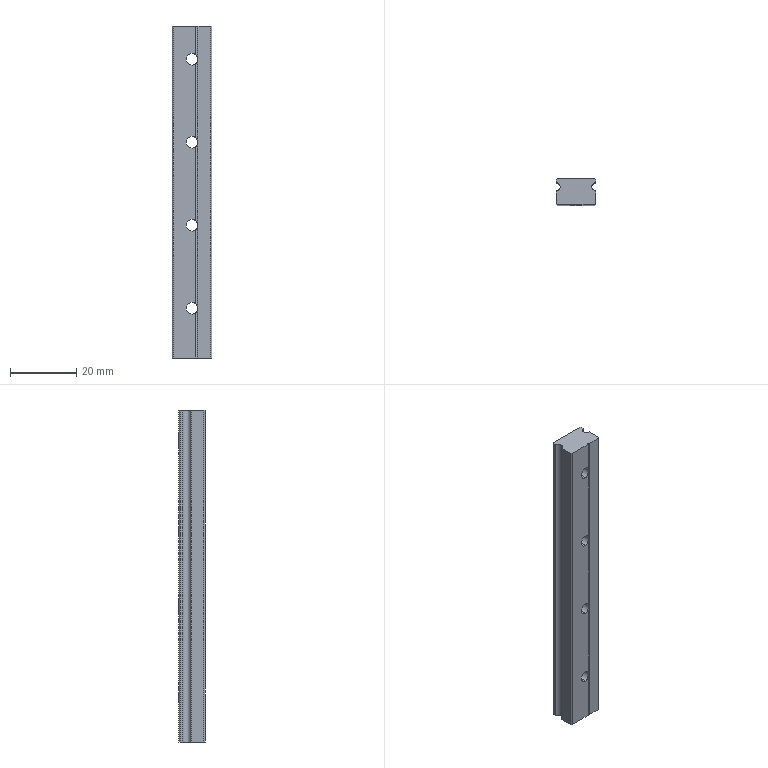Part | SolidWorks | features ICE 3, BaseBody 1 | 1 solid | 37 faces | box 12 x 8 x 100 mm | volume 8420 mm3 | cylinder 20 | plane 17 | commonest cylinder face diameters 3.5 x8 6 x8 2.5 x3 0.6 x1
STEP:
#1=CARTESIAN_POINT('',(0.,0.,-51.75));
#2=VERTEX_POINT('',#1);
#3=CARTESIAN_POINT('',(0.,0.,-48.25));
#4=VERTEX_POINT('',#3);
#5=CARTESIAN_POINT('',(0.,0.,-50.));
#6=DIRECTION('',(0.,1.,0.));
#7=DIRECTION('',(0.,0.,1.));
#8=AXIS2_PLACEMENT_3D('',#5,#6,#7);
#9=CIRCLE('',#8,1.75);
#10=EDGE_CURVE('',#2,#4,#9,.T.);
#11=ORIENTED_EDGE('',*,*,#10,.F.);
#12=CARTESIAN_POINT('',(0.,3.5,-51.75));
#13=VERTEX_POINT('',#12);
#14=CARTESIAN_POINT('',(0.,-0.006662,-51.75));
#15=DIRECTION('',(0.,1.,0.));
#16=VECTOR('',#15,1000.);
#17=LINE('',#14,#16);
#18=EDGE_CURVE('',#2,#13,#17,.T.);
#19=ORIENTED_EDGE('',*,*,#18,.T.);
#20=CARTESIAN_POINT('',(0.,3.5,-48.25));
#21=VERTEX_POINT('',#20);
#22=CARTESIAN_POINT('',(0.,3.5,-50.));
#23=DIRECTION('',(0.,1.,0.));
#24=DIRECTION('',(0.,0.,1.));
#25=AXIS2_PLACEMENT_3D('',#22,#23,#24);
#26=CIRCLE('',#25,1.75);
#27=EDGE_CURVE('',#13,#21,#26,.T.);
#28=ORIENTED_EDGE('',*,*,#27,.T.);
#29=CARTESIAN_POINT('',(0.,-0.006662,-48.25));
#30=DIRECTION('',(0.,1.,0.));
#31=VECTOR('',#30,1000.);
#32=LINE('',#29,#31);
#33=EDGE_CURVE('',#4,#21,#32,.T.);
#34=ORIENTED_EDGE('',*,*,#33,.F.);
#35=EDGE_LOOP('',(#11,#19,#28,#34));
#36=FACE_OUTER_BOUND('',#35,.T.);
#37=CARTESIAN_POINT('',(0.,-0.006662,-50.));
#38=DIRECTION('',(0.,1.,0.));
#39=DIRECTION('',(0.,0.,1.));
#40=AXIS2_PLACEMENT_3D('',#37,#38,#39);
#41=CYLINDRICAL_SURFACE('',#40,1.75);
#42=ADVANCED_FACE('',(#36),#41,.F.);
#43=CARTESIAN_POINT('',(0.,3.5,-53.));
#44=VERTEX_POINT('',#43);
#45=CARTESIAN_POINT('',(0.,3.5,-47.));
#46=VERTEX_POINT('',#45);
#47=CARTESIAN_POINT('',(0.,3.5,-50.));
#48=DIRECTION('',(0.,1.,0.));
#49=DIRECTION('',(0.,0.,1.));
#50=AXIS2_PLACEMENT_3D('',#47,#48,#49);
#51=CIRCLE('',#50,3.);
#52=EDGE_CURVE('',#44,#46,#51,.T.);
#53=ORIENTED_EDGE('',*,*,#52,.F.);
#54=CARTESIAN_POINT('',(0.,8.,-53.));
#55=VERTEX_POINT('',#54);
#56=CARTESIAN_POINT('',(0.,3.5,-53.));
#57=DIRECTION('',(0.,1.,0.));
#58=VECTOR('',#57,1000.);
#59=LINE('',#56,#58);
#60=EDGE_CURVE('',#44,#55,#59,.T.);
#61=ORIENTED_EDGE('',*,*,#60,.T.);
#62=CARTESIAN_POINT('',(0.,8.,-47.));
#63=VERTEX_POINT('',#62);
#64=CARTESIAN_POINT('',(0.,8.,-50.));
#65=DIRECTION('',(0.,1.,0.));
#66=DIRECTION('',(0.,0.,1.));
#67=AXIS2_PLACEMENT_3D('',#64,#65,#66);
#68=CIRCLE('',#67,3.);
#69=EDGE_CURVE('',#55,#63,#68,.T.);
#70=ORIENTED_EDGE('',*,*,#69,.T.);
#71=CARTESIAN_POINT('',(0.,3.5,-47.));
#72=DIRECTION('',(0.,1.,0.));
#73=VECTOR('',#72,1000.);
#74=LINE('',#71,#73);
#75=EDGE_CURVE('',#46,#63,#74,.T.);
#76=ORIENTED_EDGE('',*,*,#75,.F.);
#77=EDGE_LOOP('',(#53,#61,#70,#76));
#78=FACE_OUTER_BOUND('',#77,.T.);
#79=CARTESIAN_POINT('',(0.,3.5,-50.));
#80=DIRECTION('',(0.,1.,0.));
#81=DIRECTION('',(0.,0.,1.));
#82=AXIS2_PLACEMENT_3D('',#79,#80,#81);
#83=CYLINDRICAL_SURFACE('',#82,3.);
#84=ADVANCED_FACE('',(#78),#83,.F.);
#85=CARTESIAN_POINT('',(0.,3.5,1.75));
#86=VERTEX_POINT('',#85);
#87=CARTESIAN_POINT('',(0.,3.5,-1.75));
#88=VERTEX_POINT('',#87);
#89=CARTESIAN_POINT('',(0.,3.5,0.));
#90=DIRECTION('',(0.,-1.,0.));
#91=DIRECTION('',(0.,0.,-1.));
#92=AXIS2_PLACEMENT_3D('',#89,#90,#91);
#93=CIRCLE('',#92,1.75);
#94=EDGE_CURVE('',#86,#88,#93,.T.);
#95=ORIENTED_EDGE('',*,*,#94,.F.);
#96=CARTESIAN_POINT('',(0.,0.,1.75));
#97=VERTEX_POINT('',#96);
#98=CARTESIAN_POINT('',(0.,-8.977,1.75));
#99=DIRECTION('',(0.,-1.,0.));
#100=VECTOR('',#99,1000.);
#101=LINE('',#98,#100);
#102=EDGE_CURVE('',#86,#97,#101,.T.);
#103=ORIENTED_EDGE('',*,*,#102,.T.);
#104=CARTESIAN_POINT('',(0.,0.,-1.75));
#105=VERTEX_POINT('',#104);
#106=CARTESIAN_POINT('',(0.,0.,0.));
#107=DIRECTION('',(0.,1.,0.));
#108=DIRECTION('',(0.,0.,1.));
#109=AXIS2_PLACEMENT_3D('',#106,#107,#108);
#110=CIRCLE('',#109,1.75);
#111=EDGE_CURVE('',#105,#97,#110,.T.);
#112=ORIENTED_EDGE('',*,*,#111,.F.);
#113=CARTESIAN_POINT('',(0.,-8.977,-1.75));
#114=DIRECTION('',(0.,-1.,0.));
#115=VECTOR('',#114,1000.);
#116=LINE('',#113,#115);
#117=EDGE_CURVE('',#88,#105,#116,.T.);
#118=ORIENTED_EDGE('',*,*,#117,.F.);
#119=EDGE_LOOP('',(#95,#103,#112,#118));
#120=FACE_OUTER_BOUND('',#119,.T.);
#121=CARTESIAN_POINT('',(0.,-8.977,0.));
#122=DIRECTION('',(0.,-1.,0.));
#123=DIRECTION('',(0.,0.,-1.));
#124=AXIS2_PLACEMENT_3D('',#121,#122,#123);
#125=CYLINDRICAL_SURFACE('',#124,1.75);
#126=ADVANCED_FACE('',(#120),#125,.F.);
#127=CARTESIAN_POINT('',(0.,8.,28.));
#128=VERTEX_POINT('',#127);
#129=CARTESIAN_POINT('',(0.,8.,22.));
#130=VERTEX_POINT('',#129);
#131=CARTESIAN_POINT('',(0.,8.,25.));
#132=DIRECTION('',(0.,-1.,0.));
#133=DIRECTION('',(0.,0.,-1.));
#134=AXIS2_PLACEMENT_3D('',#131,#132,#133);
#135=CIRCLE('',#134,3.);
#136=EDGE_CURVE('',#128,#130,#135,.T.);
#137=ORIENTED_EDGE('',*,*,#136,.F.);
#138=CARTESIAN_POINT('',(0.,3.5,28.));
#139=VERTEX_POINT('',#138);
#140=CARTESIAN_POINT('',(0.,8.,28.));
#141=DIRECTION('',(0.,-1.,0.));
#142=VECTOR('',#141,1000.);
#143=LINE('',#140,#142);
#144=EDGE_CURVE('',#128,#139,#143,.T.);
#145=ORIENTED_EDGE('',*,*,#144,.T.);
#146=CARTESIAN_POINT('',(0.,3.5,22.));
#147=VERTEX_POINT('',#146);
#148=CARTESIAN_POINT('',(0.,3.5,25.));
#149=DIRECTION('',(0.,1.,0.));
#150=DIRECTION('',(-1.,0.,0.));
#151=AXIS2_PLACEMENT_3D('',#148,#149,#150);
#152=CIRCLE('',#151,3.);
#153=EDGE_CURVE('',#147,#139,#152,.T.);
#154=ORIENTED_EDGE('',*,*,#153,.F.);
#155=CARTESIAN_POINT('',(0.,8.,22.));
#156=DIRECTION('',(0.,-1.,0.));
#157=VECTOR('',#156,1000.);
#158=LINE('',#155,#157);
#159=EDGE_CURVE('',#130,#147,#158,.T.);
#160=ORIENTED_EDGE('',*,*,#159,.F.);
#161=EDGE_LOOP('',(#137,#145,#154,#160));
#162=FACE_OUTER_BOUND('',#161,.T.);
#163=CARTESIAN_POINT('',(0.,8.,25.));
#164=DIRECTION('',(0.,-1.,0.));
#165=DIRECTION('',(0.,0.,-1.));
#166=AXIS2_PLACEMENT_3D('',#163,#164,#165);
#167=CYLINDRICAL_SURFACE('',#166,3.);
#168=ADVANCED_FACE('',(#162),#167,.F.);
#169=CARTESIAN_POINT('',(4.75,5.5,35.));
#170=VERTEX_POINT('',#169);
#171=CARTESIAN_POINT('',(6.,6.75,35.));
#172=VERTEX_POINT('',#171);
#173=CARTESIAN_POINT('',(6.,5.5,35.));
#174=DIRECTION('',(0.,0.,-1.));
#175=DIRECTION('',(0.,-1.,0.));
#176=AXIS2_PLACEMENT_3D('',#173,#174,#175);
#177=CIRCLE('',#176,1.25);
#178=EDGE_CURVE('',#170,#172,#177,.T.);
#179=ORIENTED_EDGE('',*,*,#178,.F.);
#180=CARTESIAN_POINT('',(4.75,5.5,-65.));
#181=VERTEX_POINT('',#180);
#182=CARTESIAN_POINT('',(4.75,5.5,35.));
#183=DIRECTION('',(0.,0.,-1.));
#184=VECTOR('',#183,1000.);
#185=LINE('',#182,#184);
#186=EDGE_CURVE('',#170,#181,#185,.T.);
#187=ORIENTED_EDGE('',*,*,#186,.T.);
#188=CARTESIAN_POINT('',(6.,6.75,-65.));
#189=VERTEX_POINT('',#188);
#190=CARTESIAN_POINT('',(6.,5.5,-65.));
#191=DIRECTION('',(0.,0.,1.));
#192=DIRECTION('',(-1.,0.,0.));
#193=AXIS2_PLACEMENT_3D('',#190,#191,#192);
#194=CIRCLE('',#193,1.25);
#195=EDGE_CURVE('',#189,#181,#194,.T.);
#196=ORIENTED_EDGE('',*,*,#195,.F.);
#197=CARTESIAN_POINT('',(6.,6.75,-35.));
#198=DIRECTION('',(0.,0.,1.));
#199=VECTOR('',#198,1000.);
#200=LINE('',#197,#199);
#201=EDGE_CURVE('',#189,#172,#200,.T.);
#202=ORIENTED_EDGE('',*,*,#201,.T.);
#203=EDGE_LOOP('',(#179,#187,#196,#202));
#204=FACE_OUTER_BOUND('',#203,.T.);
#205=CARTESIAN_POINT('',(6.,5.5,35.));
#206=DIRECTION('',(0.,0.,-1.));
#207=DIRECTION('',(-1.,0.,0.));
#208=AXIS2_PLACEMENT_3D('',#205,#206,#207);
#209=CYLINDRICAL_SURFACE('',#208,1.25);
#210=ADVANCED_FACE('',(#204),#209,.F.);
#211=CARTESIAN_POINT('',(0.,8.,-22.));
#212=VERTEX_POINT('',#211);
#213=CARTESIAN_POINT('',(0.,8.,-28.));
#214=VERTEX_POINT('',#213);
#215=CARTESIAN_POINT('',(0.,8.,-25.));
#216=DIRECTION('',(0.,-1.,0.));
#217=DIRECTION('',(0.,0.,-1.));
#218=AXIS2_PLACEMENT_3D('',#215,#216,#217);
#219=CIRCLE('',#218,3.);
#220=EDGE_CURVE('',#212,#214,#219,.T.);
#221=ORIENTED_EDGE('',*,*,#220,.F.);
#222=CARTESIAN_POINT('',(0.,3.5,-22.));
#223=VERTEX_POINT('',#222);
#224=CARTESIAN_POINT('',(0.,8.,-22.));
#225=DIRECTION('',(0.,-1.,0.));
#226=VECTOR('',#225,1000.);
#227=LINE('',#224,#226);
#228=EDGE_CURVE('',#212,#223,#227,.T.);
#229=ORIENTED_EDGE('',*,*,#228,.T.);
#230=CARTESIAN_POINT('',(0.,3.5,-28.));
#231=VERTEX_POINT('',#230);
#232=CARTESIAN_POINT('',(0.,3.5,-25.));
#233=DIRECTION('',(0.,1.,0.));
#234=DIRECTION('',(-1.,0.,0.));
#235=AXIS2_PLACEMENT_3D('',#232,#233,#234);
#236=CIRCLE('',#235,3.);
#237=EDGE_CURVE('',#231,#223,#236,.T.);
#238=ORIENTED_EDGE('',*,*,#237,.F.);
#239=CARTESIAN_POINT('',(0.,8.,-28.));
#240=DIRECTION('',(0.,-1.,0.));
#241=VECTOR('',#240,1000.);
#242=LINE('',#239,#241);
#243=EDGE_CURVE('',#214,#231,#242,.T.);
#244=ORIENTED_EDGE('',*,*,#243,.F.);
#245=EDGE_LOOP('',(#221,#229,#238,#244));
#246=FACE_OUTER_BOUND('',#245,.T.);
#247=CARTESIAN_POINT('',(0.,8.,-25.));
#248=DIRECTION('',(0.,-1.,0.));
#249=DIRECTION('',(0.,0.,-1.));
#250=AXIS2_PLACEMENT_3D('',#247,#248,#249);
#251=CYLINDRICAL_SURFACE('',#250,3.);
#252=ADVANCED_FACE('',(#246),#251,.F.);
#253=CARTESIAN_POINT('',(0.,8.,3.));
#254=VERTEX_POINT('',#253);
#255=CARTESIAN_POINT('',(0.,8.,-3.));
#256=VERTEX_POINT('',#255);
#257=CARTESIAN_POINT('',(0.,8.,0.));
#258=DIRECTION('',(0.,-1.,0.));
#259=DIRECTION('',(0.,0.,-1.));
#260=AXIS2_PLACEMENT_3D('',#257,#258,#259);
#261=CIRCLE('',#260,3.);
#262=EDGE_CURVE('',#254,#256,#261,.T.);
#263=ORIENTED_EDGE('',*,*,#262,.F.);
#264=CARTESIAN_POINT('',(0.,3.5,3.));
#265=VERTEX_POINT('',#264);
#266=CARTESIAN_POINT('',(0.,8.,3.));
#267=DIRECTION('',(0.,-1.,0.));
#268=VECTOR('',#267,1000.);
#269=LINE('',#266,#268);
#270=EDGE_CURVE('',#254,#265,#269,.T.);
#271=ORIENTED_EDGE('',*,*,#270,.T.);
#272=CARTESIAN_POINT('',(0.,3.5,-3.));
#273=VERTEX_POINT('',#272);
#274=CARTESIAN_POINT('',(0.,3.5,0.));
#275=DIRECTION('',(0.,1.,0.));
#276=DIRECTION('',(-1.,0.,0.));
#277=AXIS2_PLACEMENT_3D('',#274,#275,#276);
#278=CIRCLE('',#277,3.);
#279=EDGE_CURVE('',#273,#265,#278,.T.);
#280=ORIENTED_EDGE('',*,*,#279,.F.);
#281=CARTESIAN_POINT('',(0.,8.,-3.));
#282=DIRECTION('',(0.,-1.,0.));
#283=VECTOR('',#282,1000.);
#284=LINE('',#281,#283);
#285=EDGE_CURVE('',#256,#273,#284,.T.);
#286=ORIENTED_EDGE('',*,*,#285,.F.);
#287=EDGE_LOOP('',(#263,#271,#280,#286));
#288=FACE_OUTER_BOUND('',#287,.T.);
#289=CARTESIAN_POINT('',(0.,8.,0.));
#290=DIRECTION('',(0.,-1.,0.));
#291=DIRECTION('',(0.,0.,-1.));
#292=AXIS2_PLACEMENT_3D('',#289,#290,#291);
#293=CYLINDRICAL_SURFACE('',#292,3.);
#294=ADVANCED_FACE('',(#288),#293,.F.);
#295=CARTESIAN_POINT('',(0.,3.5,26.75));
#296=VERTEX_POINT('',#295);
#297=CARTESIAN_POINT('',(0.,3.5,23.25));
#298=VERTEX_POINT('',#297);
#299=CARTESIAN_POINT('',(0.,3.5,25.));
#300=DIRECTION('',(0.,-1.,0.));
#301=DIRECTION('',(0.,0.,-1.));
#302=AXIS2_PLACEMENT_3D('',#299,#300,#301);
#303=CIRCLE('',#302,1.75);
#304=EDGE_CURVE('',#296,#298,#303,.T.);
#305=ORIENTED_EDGE('',*,*,#304,.F.);
#306=CARTESIAN_POINT('',(0.,0.,26.75));
#307=VERTEX_POINT('',#306);
#308=CARTESIAN_POINT('',(0.,-8.977,26.75));
#309=DIRECTION('',(0.,-1.,0.));
#310=VECTOR('',#309,1000.);
#311=LINE('',#308,#310);
#312=EDGE_CURVE('',#296,#307,#311,.T.);
#313=ORIENTED_EDGE('',*,*,#312,.T.);
#314=CARTESIAN_POINT('',(0.,0.,23.25));
#315=VERTEX_POINT('',#314);
#316=CARTESIAN_POINT('',(0.,0.,25.));
#317=DIRECTION('',(0.,1.,0.));
#318=DIRECTION('',(0.,0.,1.));
#319=AXIS2_PLACEMENT_3D('',#316,#317,#318);
#320=CIRCLE('',#319,1.75);
#321=EDGE_CURVE('',#315,#307,#320,.T.);
#322=ORIENTED_EDGE('',*,*,#321,.F.);
#323=CARTESIAN_POINT('',(0.,-8.977,23.25));
#324=DIRECTION('',(0.,-1.,0.));
#325=VECTOR('',#324,1000.);
#326=LINE('',#323,#325);
#327=EDGE_CURVE('',#298,#315,#326,.T.);
#328=ORIENTED_EDGE('',*,*,#327,.F.);
#329=EDGE_LOOP('',(#305,#313,#322,#328));
#330=FACE_OUTER_BOUND('',#329,.T.);
#331=CARTESIAN_POINT('',(0.,-8.977,25.));
#332=DIRECTION('',(0.,-1.,0.));
#333=DIRECTION('',(0.,0.,-1.));
#334=AXIS2_PLACEMENT_3D('',#331,#332,#333);
#335=CYLINDRICAL_SURFACE('',#334,1.75);
#336=ADVANCED_FACE('',(#330),#335,.F.);
#337=CARTESIAN_POINT('',(0.,3.5,-23.25));
#338=VERTEX_POINT('',#337);
#339=CARTESIAN_POINT('',(0.,3.5,-26.75));
#340=VERTEX_POINT('',#339);
#341=CARTESIAN_POINT('',(0.,3.5,-25.));
#342=DIRECTION('',(0.,-1.,0.));
#343=DIRECTION('',(0.,0.,-1.));
#344=AXIS2_PLACEMENT_3D('',#341,#342,#343);
#345=CIRCLE('',#344,1.75);
#346=EDGE_CURVE('',#338,#340,#345,.T.);
#347=ORIENTED_EDGE('',*,*,#346,.F.);
#348=CARTESIAN_POINT('',(0.,0.,-23.25));
#349=VERTEX_POINT('',#348);
#350=CARTESIAN_POINT('',(0.,-8.977,-23.25));
#351=DIRECTION('',(0.,-1.,0.));
#352=VECTOR('',#351,1000.);
#353=LINE('',#350,#352);
#354=EDGE_CURVE('',#338,#349,#353,.T.);
#355=ORIENTED_EDGE('',*,*,#354,.T.);
#356=CARTESIAN_POINT('',(0.,0.,-26.75));
#357=VERTEX_POINT('',#356);
#358=CARTESIAN_POINT('',(0.,0.,-25.));
#359=DIRECTION('',(0.,1.,0.));
#360=DIRECTION('',(0.,0.,1.));
#361=AXIS2_PLACEMENT_3D('',#358,#359,#360);
#362=CIRCLE('',#361,1.75);
#363=EDGE_CURVE('',#357,#349,#362,.T.);
#364=ORIENTED_EDGE('',*,*,#363,.F.);
#365=CARTESIAN_POINT('',(0.,-8.977,-26.75));
#366=DIRECTION('',(0.,-1.,0.));
#367=VECTOR('',#366,1000.);
#368=LINE('',#365,#367);
#369=EDGE_CURVE('',#340,#357,#368,.T.);
#370=ORIENTED_EDGE('',*,*,#369,.F.);
#371=EDGE_LOOP('',(#347,#355,#364,#370));
#372=FACE_OUTER_BOUND('',#371,.T.);
#373=CARTESIAN_POINT('',(0.,-8.977,-25.));
#374=DIRECTION('',(0.,-1.,0.));
#375=DIRECTION('',(0.,0.,-1.));
#376=AXIS2_PLACEMENT_3D('',#373,#374,#375);
#377=CYLINDRICAL_SURFACE('',#376,1.75);
#378=ADVANCED_FACE('',(#372),#377,.F.);
#379=ORIENTED_EDGE('',*,*,#354,.F.);
#380=CARTESIAN_POINT('',(0.,3.5,-25.));
#381=DIRECTION('',(0.,-1.,0.));
#382=DIRECTION('',(0.,0.,-1.));
#383=AXIS2_PLACEMENT_3D('',#380,#381,#382);
#384=CIRCLE('',#383,1.75);
#385=EDGE_CURVE('',#340,#338,#384,.T.);
#386=ORIENTED_EDGE('',*,*,#385,.F.);
#387=ORIENTED_EDGE('',*,*,#369,.T.);
#388=CARTESIAN_POINT('',(1.2,0.,-26.274));
#389=VERTEX_POINT('',#388);
#390=CARTESIAN_POINT('',(0.,0.,-25.));
#391=DIRECTION('',(0.,1.,0.));
#392=DIRECTION('',(0.,0.,1.));
#393=AXIS2_PLACEMENT_3D('',#390,#391,#392);
#394=CIRCLE('',#393,1.75);
#395=EDGE_CURVE('',#389,#357,#394,.T.);
#396=ORIENTED_EDGE('',*,*,#395,.F.);
#397=CARTESIAN_POINT('',(1.2,0.,-23.726));
#398=VERTEX_POINT('',#397);
#399=CARTESIAN_POINT('',(1.2,0.,-26.274));
#400=CARTESIAN_POINT('',(1.2,0.02075,-26.274));
#401=CARTESIAN_POINT('',(1.202,0.04091,-26.272));
#402=CARTESIAN_POINT('',(1.21,0.08005,-26.264));
#403=CARTESIAN_POINT('',(1.216,0.09786,-26.259));
#404=CARTESIAN_POINT('',(1.241,0.1565,-26.234));
#405=CARTESIAN_POINT('',(1.265,0.1906,-26.21));
#406=CARTESIAN_POINT('',(1.321,0.2436,-26.149));
#407=CARTESIAN_POINT('',(1.352,0.2638,-26.112));
#408=CARTESIAN_POINT('',(1.403,0.2845,-26.047));
#409=CARTESIAN_POINT('',(1.42,0.2898,-26.023));
#410=CARTESIAN_POINT('',(1.446,0.2954,-25.985));
#411=CARTESIAN_POINT('',(1.46,0.2976,-25.966));
#412=CARTESIAN_POINT('',(1.473,0.2988,-25.945));
#413=CARTESIAN_POINT('',(1.482,0.2995,-25.931));
#414=CARTESIAN_POINT('',(1.488,0.2998,-25.922));
#415=CARTESIAN_POINT('',(1.52,0.3007,-25.87));
#416=CARTESIAN_POINT('',(1.55,0.2969,-25.815));
#417=CARTESIAN_POINT('',(1.595,0.2843,-25.72));
#418=CARTESIAN_POINT('',(1.61,0.2789,-25.686));
#419=CARTESIAN_POINT('',(1.639,0.2659,-25.613));
#420=CARTESIAN_POINT('',(1.654,0.2578,-25.573));
#421=CARTESIAN_POINT('',(1.679,0.241,-25.494));
#422=CARTESIAN_POINT('',(1.696,0.2284,-25.435));
#423=CARTESIAN_POINT('',(1.709,0.2156,-25.375));
#424=CARTESIAN_POINT('',(1.718,0.2071,-25.335));
#425=CARTESIAN_POINT('',(1.721,0.2032,-25.317));
#426=CARTESIAN_POINT('',(1.733,0.1892,-25.25));
#427=CARTESIAN_POINT('',(1.741,0.1782,-25.183));
#428=CARTESIAN_POINT('',(1.746,0.1718,-25.116));
#429=CARTESIAN_POINT('',(1.749,0.1686,-25.071));
#430=CARTESIAN_POINT('',(1.749,0.1674,-25.047));
#431=CARTESIAN_POINT('',(1.75,0.1657,-24.985));
#432=CARTESIAN_POINT('',(1.75,0.167,-24.941));
#433=CARTESIAN_POINT('',(1.746,0.1726,-24.873));
#434=CARTESIAN_POINT('',(1.743,0.1762,-24.839));
#435=CARTESIAN_POINT('',(1.738,0.1821,-24.797));
#436=CARTESIAN_POINT('',(1.736,0.1854,-24.776));
#437=CARTESIAN_POINT('',(1.734,0.187,-24.767));
#438=CARTESIAN_POINT('',(1.734,0.188,-24.761));
#439=CARTESIAN_POINT('',(1.733,0.1889,-24.756));
#440=CARTESIAN_POINT('',(1.73,0.192,-24.738));
#441=CARTESIAN_POINT('',(1.726,0.1978,-24.709));
#442=CARTESIAN_POINT('',(1.714,0.2107,-24.646));
#443=CARTESIAN_POINT('',(1.709,0.2157,-24.623));
#444=CARTESIAN_POINT('',(1.699,0.2243,-24.582));
#445=CARTESIAN_POINT('',(1.694,0.2289,-24.561));
#446=CARTESIAN_POINT('',(1.687,0.2347,-24.534));
#447=CARTESIAN_POINT('',(1.684,0.2373,-24.522));
#448=CARTESIAN_POINT('',(1.681,0.239,-24.514));
#449=CARTESIAN_POINT('',(1.68,0.2402,-24.509));
#450=CARTESIAN_POINT('',(1.653,0.2604,-24.417));
#451=CARTESIAN_POINT('',(1.622,0.2752,-24.339));
#452=CARTESIAN_POINT('',(1.576,0.29,-24.238));
#453=CARTESIAN_POINT('',(1.56,0.2937,-24.207));
#454=CARTESIAN_POINT('',(1.538,0.2974,-24.164));
#455=CARTESIAN_POINT('',(1.526,0.2988,-24.144));
#456=CARTESIAN_POINT('',(1.515,0.2996,-24.125));
#457=CARTESIAN_POINT('',(1.508,0.2999,-24.112));
#458=CARTESIAN_POINT('',(1.506,0.3,-24.108));
#459=CARTESIAN_POINT('',(1.464,0.3001,-24.039));
#460=CARTESIAN_POINT('',(1.427,0.2936,-23.986));
#461=CARTESIAN_POINT('',(1.358,0.2669,-23.894));
#462=CARTESIAN_POINT('',(1.326,0.2475,-23.857));
#463=CARTESIAN_POINT('',(1.281,0.2065,-23.808));
#464=CARTESIAN_POINT('',(1.268,0.1912,-23.794));
#465=CARTESIAN_POINT('',(1.244,0.1575,-23.769));
#466=CARTESIAN_POINT('',(1.233,0.1376,-23.758));
#467=CARTESIAN_POINT('',(1.208,0.08193,-23.734));
#468=CARTESIAN_POINT('',(1.2,0.04225,-23.726));
#469=CARTESIAN_POINT('',(1.2,0.,-23.726));
#470=B_SPLINE_CURVE_WITH_KNOTS('',3,(#399,#400,#401,#402,#403,#404,#405,#406,#407,#408,#409,#410,#411,#412,#413,#414,#415,#416,#417,#418,#419,#420,#421,#422,#423,#424,#425,#426,#427,#428,#429,#430,#431,#432,#433,#434,#435,#436,#437,#438,#439,#440,#441,#442,#443,#444,#445,#446,#447,#448,#449,#450,#451,#452,#453,#454,#455,#456,#457,#458,#459,#460,#461,#462,#463,#464,#465,#466,#467,#468,#469),.UNSPECIFIED.,.F.,.F.,(4,2,2,2,2,2,1,2,2,2,2,2,1,2,2,1,2,2,2,1,1,1,2,2,2,2,1,1,2,2,2,2,1,2,2,2,2,2,2,4),(0.,0.03125,0.0625,0.125,0.1875,0.2187,0.2344,0.2422,0.25,0.3125,0.3437,0.375,0.4062,0.4219,0.4375,0.4687,0.4844,0.5,0.5312,0.5469,0.5547,0.5586,0.5605,0.5625,0.5937,0.6094,0.6172,0.6211,0.623,0.625,0.6875,0.7187,0.7344,0.7422,0.75,0.8125,0.875,0.9062,0.9375,1.),.UNSPECIFIED.);
#471=EDGE_CURVE('',#389,#398,#470,.T.);
#472=ORIENTED_EDGE('',*,*,#471,.T.);
#473=CARTESIAN_POINT('',(0.,0.,-25.));
#474=DIRECTION('',(0.,1.,0.));
#475=DIRECTION('',(0.,0.,1.));
#476=AXIS2_PLACEMENT_3D('',#473,#474,#475);
#477=CIRCLE('',#476,1.75);
#478=EDGE_CURVE('',#349,#398,#477,.T.);
#479=ORIENTED_EDGE('',*,*,#478,.F.);
#480=EDGE_LOOP('',(#379,#386,#387,#396,#472,#479));
#481=FACE_OUTER_BOUND('',#480,.T.);
#482=CARTESIAN_POINT('',(0.,-8.977,-25.));
#483=DIRECTION('',(0.,-1.,0.));
#484=DIRECTION('',(0.,0.,-1.));
#485=AXIS2_PLACEMENT_3D('',#482,#483,#484);
#486=CYLINDRICAL_SURFACE('',#485,1.75);
#487=ADVANCED_FACE('',(#481),#486,.F.);
#488=ORIENTED_EDGE('',*,*,#312,.F.);
#489=CARTESIAN_POINT('',(0.,3.5,25.));
#490=DIRECTION('',(0.,-1.,0.));
#491=DIRECTION('',(0.,0.,-1.));
#492=AXIS2_PLACEMENT_3D('',#489,#490,#491);
#493=CIRCLE('',#492,1.75);
#494=EDGE_CURVE('',#298,#296,#493,.T.);
#495=ORIENTED_EDGE('',*,*,#494,.F.);
#496=ORIENTED_EDGE('',*,*,#327,.T.);
#497=CARTESIAN_POINT('',(1.2,0.,23.726));
#498=VERTEX_POINT('',#497);
#499=CARTESIAN_POINT('',(0.,0.,25.));
#500=DIRECTION('',(0.,1.,0.));
#501=DIRECTION('',(0.,0.,1.));
#502=AXIS2_PLACEMENT_3D('',#499,#500,#501);
#503=CIRCLE('',#502,1.75);
#504=EDGE_CURVE('',#498,#315,#503,.T.);
#505=ORIENTED_EDGE('',*,*,#504,.F.);
#506=CARTESIAN_POINT('',(1.2,0.,26.274));
#507=VERTEX_POINT('',#506);
#508=CARTESIAN_POINT('',(1.2,0.,23.726));
#509=CARTESIAN_POINT('',(1.2,0.02075,23.726));
#510=CARTESIAN_POINT('',(1.202,0.04091,23.728));
#511=CARTESIAN_POINT('',(1.21,0.08005,23.736));
#512=CARTESIAN_POINT('',(1.216,0.09786,23.741));
#513=CARTESIAN_POINT('',(1.241,0.1565,23.766));
#514=CARTESIAN_POINT('',(1.265,0.1906,23.79));
#515=CARTESIAN_POINT('',(1.321,0.2436,23.851));
#516=CARTESIAN_POINT('',(1.352,0.2638,23.888));
#517=CARTESIAN_POINT('',(1.403,0.2845,23.953));
#518=CARTESIAN_POINT('',(1.42,0.2898,23.977));
#519=CARTESIAN_POINT('',(1.446,0.2954,24.015));
#520=CARTESIAN_POINT('',(1.46,0.2976,24.034));
#521=CARTESIAN_POINT('',(1.473,0.2988,24.055));
#522=CARTESIAN_POINT('',(1.482,0.2995,24.069));
#523=CARTESIAN_POINT('',(1.488,0.2998,24.078));
#524=CARTESIAN_POINT('',(1.52,0.3007,24.13));
#525=CARTESIAN_POINT('',(1.55,0.2969,24.185));
#526=CARTESIAN_POINT('',(1.595,0.2843,24.28));
#527=CARTESIAN_POINT('',(1.61,0.2789,24.314));
#528=CARTESIAN_POINT('',(1.639,0.2659,24.387));
#529=CARTESIAN_POINT('',(1.654,0.2578,24.427));
#530=CARTESIAN_POINT('',(1.679,0.241,24.506));
#531=CARTESIAN_POINT('',(1.696,0.2284,24.565));
#532=CARTESIAN_POINT('',(1.709,0.2156,24.625));
#533=CARTESIAN_POINT('',(1.718,0.2071,24.665));
#534=CARTESIAN_POINT('',(1.721,0.2032,24.683));
#535=CARTESIAN_POINT('',(1.733,0.1892,24.75));
#536=CARTESIAN_POINT('',(1.741,0.1782,24.817));
#537=CARTESIAN_POINT('',(1.746,0.1718,24.884));
#538=CARTESIAN_POINT('',(1.749,0.1686,24.929));
#539=CARTESIAN_POINT('',(1.749,0.1674,24.953));
#540=CARTESIAN_POINT('',(1.75,0.1657,25.015));
#541=CARTESIAN_POINT('',(1.75,0.167,25.059));
#542=CARTESIAN_POINT('',(1.746,0.1726,25.127));
#543=CARTESIAN_POINT('',(1.743,0.1762,25.161));
#544=CARTESIAN_POINT('',(1.738,0.1821,25.203));
#545=CARTESIAN_POINT('',(1.736,0.1854,25.224));
#546=CARTESIAN_POINT('',(1.734,0.187,25.233));
#547=CARTESIAN_POINT('',(1.734,0.188,25.239));
#548=CARTESIAN_POINT('',(1.733,0.1889,25.244));
#549=CARTESIAN_POINT('',(1.73,0.192,25.262));
#550=CARTESIAN_POINT('',(1.726,0.1978,25.291));
#551=CARTESIAN_POINT('',(1.714,0.2107,25.354));
#552=CARTESIAN_POINT('',(1.709,0.2157,25.377));
#553=CARTESIAN_POINT('',(1.699,0.2243,25.418));
#554=CARTESIAN_POINT('',(1.694,0.2289,25.439));
#555=CARTESIAN_POINT('',(1.687,0.2347,25.466));
#556=CARTESIAN_POINT('',(1.684,0.2373,25.478));
#557=CARTESIAN_POINT('',(1.681,0.239,25.486));
#558=CARTESIAN_POINT('',(1.68,0.2402,25.491));
#559=CARTESIAN_POINT('',(1.653,0.2604,25.583));
#560=CARTESIAN_POINT('',(1.622,0.2752,25.661));
#561=CARTESIAN_POINT('',(1.576,0.29,25.762));
#562=CARTESIAN_POINT('',(1.56,0.2937,25.793));
#563=CARTESIAN_POINT('',(1.538,0.2974,25.836));
#564=CARTESIAN_POINT('',(1.526,0.2988,25.856));
#565=CARTESIAN_POINT('',(1.515,0.2996,25.875));
#566=CARTESIAN_POINT('',(1.508,0.2999,25.888));
#567=CARTESIAN_POINT('',(1.506,0.3,25.892));
#568=CARTESIAN_POINT('',(1.464,0.3001,25.961));
#569=CARTESIAN_POINT('',(1.427,0.2936,26.014));
#570=CARTESIAN_POINT('',(1.358,0.2669,26.106));
#571=CARTESIAN_POINT('',(1.326,0.2475,26.143));
#572=CARTESIAN_POINT('',(1.281,0.2065,26.192));
#573=CARTESIAN_POINT('',(1.268,0.1912,26.206));
#574=CARTESIAN_POINT('',(1.244,0.1575,26.231));
#575=CARTESIAN_POINT('',(1.233,0.1376,26.242));
#576=CARTESIAN_POINT('',(1.208,0.08193,26.266));
#577=CARTESIAN_POINT('',(1.2,0.04225,26.274));
#578=CARTESIAN_POINT('',(1.2,0.,26.274));
#579=B_SPLINE_CURVE_WITH_KNOTS('',3,(#508,#509,#510,#511,#512,#513,#514,#515,#516,#517,#518,#519,#520,#521,#522,#523,#524,#525,#526,#527,#528,#529,#530,#531,#532,#533,#534,#535,#536,#537,#538,#539,#540,#541,#542,#543,#544,#545,#546,#547,#548,#549,#550,#551,#552,#553,#554,#555,#556,#557,#558,#559,#560,#561,#562,#563,#564,#565,#566,#567,#568,#569,#570,#571,#572,#573,#574,#575,#576,#577,#578),.UNSPECIFIED.,.F.,.F.,(4,2,2,2,2,2,1,2,2,2,2,2,1,2,2,1,2,2,2,1,1,1,2,2,2,2,1,1,2,2,2,2,1,2,2,2,2,2,2,4),(0.,0.03125,0.0625,0.125,0.1875,0.2187,0.2344,0.2422,0.25,0.3125,0.3437,0.375,0.4062,0.4219,0.4375,0.4687,0.4844,0.5,0.5312,0.5469,0.5547,0.5586,0.5605,0.5625,0.5937,0.6094,0.6172,0.6211,0.623,0.625,0.6875,0.7187,0.7344,0.7422,0.75,0.8125,0.875,0.9062,0.9375,1.),.UNSPECIFIED.);
#580=EDGE_CURVE('',#498,#507,#579,.T.);
#581=ORIENTED_EDGE('',*,*,#580,.T.);
#582=CARTESIAN_POINT('',(0.,0.,25.));
#583=DIRECTION('',(0.,1.,0.));
#584=DIRECTION('',(0.,0.,1.));
#585=AXIS2_PLACEMENT_3D('',#582,#583,#584);
#586=CIRCLE('',#585,1.75);
#587=EDGE_CURVE('',#307,#507,#586,.T.);
#588=ORIENTED_EDGE('',*,*,#587,.F.);
#589=EDGE_LOOP('',(#488,#495,#496,#505,#581,#588));
#590=FACE_OUTER_BOUND('',#589,.T.);
#591=CARTESIAN_POINT('',(0.,-8.977,25.));
#592=DIRECTION('',(0.,-1.,0.));
#593=DIRECTION('',(0.,0.,-1.));
#594=AXIS2_PLACEMENT_3D('',#591,#592,#593);
#595=CYLINDRICAL_SURFACE('',#594,1.75);
#596=ADVANCED_FACE('',(#590),#595,.F.);
#597=ORIENTED_EDGE('',*,*,#270,.F.);
#598=CARTESIAN_POINT('',(0.,8.,0.));
#599=DIRECTION('',(0.,-1.,0.));
#600=DIRECTION('',(0.,0.,-1.));
#601=AXIS2_PLACEMENT_3D('',#598,#599,#600);
#602=CIRCLE('',#601,3.);
#603=EDGE_CURVE('',#256,#254,#602,.T.);
#604=ORIENTED_EDGE('',*,*,#603,.F.);
#605=ORIENTED_EDGE('',*,*,#285,.T.);
#606=CARTESIAN_POINT('',(0.,3.5,0.));
#607=DIRECTION('',(0.,1.,0.));
#608=DIRECTION('',(-1.,0.,0.));
#609=AXIS2_PLACEMENT_3D('',#606,#607,#608);
#610=CIRCLE('',#609,3.);
#611=EDGE_CURVE('',#265,#273,#610,.T.);
#612=ORIENTED_EDGE('',*,*,#611,.F.);
#613=EDGE_LOOP('',(#597,#604,#605,#612));
#614=FACE_OUTER_BOUND('',#613,.T.);
#615=CARTESIAN_POINT('',(0.,8.,0.));
#616=DIRECTION('',(0.,-1.,0.));
#617=DIRECTION('',(0.,0.,-1.));
#618=AXIS2_PLACEMENT_3D('',#615,#616,#617);
#619=CYLINDRICAL_SURFACE('',#618,3.);
#620=ADVANCED_FACE('',(#614),#619,.F.);
#621=ORIENTED_EDGE('',*,*,#228,.F.);
#622=CARTESIAN_POINT('',(0.,8.,-25.));
#623=DIRECTION('',(0.,-1.,0.));
#624=DIRECTION('',(0.,0.,-1.));
#625=AXIS2_PLACEMENT_3D('',#622,#623,#624);
#626=CIRCLE('',#625,3.);
#627=EDGE_CURVE('',#214,#212,#626,.T.);
#628=ORIENTED_EDGE('',*,*,#627,.F.);
#629=ORIENTED_EDGE('',*,*,#243,.T.);
#630=CARTESIAN_POINT('',(0.,3.5,-25.));
#631=DIRECTION('',(0.,1.,0.));
#632=DIRECTION('',(-1.,0.,0.));
#633=AXIS2_PLACEMENT_3D('',#630,#631,#632);
#634=CIRCLE('',#633,3.);
#635=EDGE_CURVE('',#223,#231,#634,.T.);
#636=ORIENTED_EDGE('',*,*,#635,.F.);
#637=EDGE_LOOP('',(#621,#628,#629,#636));
#638=FACE_OUTER_BOUND('',#637,.T.);
#639=CARTESIAN_POINT('',(0.,8.,-25.));
#640=DIRECTION('',(0.,-1.,0.));
#641=DIRECTION('',(0.,0.,-1.));
#642=AXIS2_PLACEMENT_3D('',#639,#640,#641);
#643=CYLINDRICAL_SURFACE('',#642,3.);
#644=ADVANCED_FACE('',(#638),#643,.F.);
#645=CARTESIAN_POINT('',(-6.,7.6,-65.));
#646=VERTEX_POINT('',#645);
#647=CARTESIAN_POINT('',(-6.,7.6,35.));
#648=VERTEX_POINT('',#647);
#649=CARTESIAN_POINT('',(-6.,7.6,-35.));
#650=DIRECTION('',(0.,0.,1.));
#651=VECTOR('',#650,1000.);
#652=LINE('',#649,#651);
#653=EDGE_CURVE('',#646,#648,#652,.T.);
#654=ORIENTED_EDGE('',*,*,#653,.F.);
#655=CARTESIAN_POINT('',(-6.,6.75,-65.));
#656=VERTEX_POINT('',#655);
#657=CARTESIAN_POINT('',(-6.,6.75,-65.));
#658=DIRECTION('',(0.,1.,0.));
#659=VECTOR('',#658,1000.);
#660=LINE('',#657,#659);
#661=EDGE_CURVE('',#656,#646,#660,.T.);
#662=ORIENTED_EDGE('',*,*,#661,.F.);
#663=CARTESIAN_POINT('',(-6.,6.75,35.));
#664=VERTEX_POINT('',#663);
#665=CARTESIAN_POINT('',(-6.,6.75,35.));
#666=DIRECTION('',(0.,0.,-1.));
#667=VECTOR('',#666,1000.);
#668=LINE('',#665,#667);
#669=EDGE_CURVE('',#664,#656,#668,.T.);
#670=ORIENTED_EDGE('',*,*,#669,.F.);
#671=CARTESIAN_POINT('',(-6.,6.75,35.));
#672=DIRECTION('',(0.,1.,0.));
#673=VECTOR('',#672,1000.);
#674=LINE('',#671,#673);
#675=EDGE_CURVE('',#664,#648,#674,.T.);
#676=ORIENTED_EDGE('',*,*,#675,.T.);
#677=EDGE_LOOP('',(#654,#662,#670,#676));
#678=FACE_OUTER_BOUND('',#677,.T.);
#679=CARTESIAN_POINT('',(-6.,8.,35.));
#680=DIRECTION('',(1.,0.,0.));
#681=DIRECTION('',(0.,1.,0.));
#682=AXIS2_PLACEMENT_3D('',#679,#680,#681);
#683=PLANE('',#682);
#684=ADVANCED_FACE('',(#678),#683,.F.);
#685=CARTESIAN_POINT('',(-5.6,8.,35.));
#686=VERTEX_POINT('',#685);
#687=CARTESIAN_POINT('',(-5.6,8.,-65.));
#688=VERTEX_POINT('',#687);
#689=CARTESIAN_POINT('',(-5.6,8.,35.));
#690=DIRECTION('',(0.,0.,-1.));
#691=VECTOR('',#690,1000.);
#692=LINE('',#689,#691);
#693=EDGE_CURVE('',#686,#688,#692,.T.);
#694=ORIENTED_EDGE('',*,*,#693,.T.);
#695=CARTESIAN_POINT('',(-6.,7.6,-65.));
#696=DIRECTION('',(0.7071,0.7071,0.));
#697=VECTOR('',#696,1000.);
#698=LINE('',#695,#697);
#699=EDGE_CURVE('',#646,#688,#698,.T.);
#700=ORIENTED_EDGE('',*,*,#699,.F.);
#701=ORIENTED_EDGE('',*,*,#653,.T.);
#702=CARTESIAN_POINT('',(-5.6,8.,35.));
#703=DIRECTION('',(-0.7071,-0.7071,0.));
#704=VECTOR('',#703,1000.);
#705=LINE('',#702,#704);
#706=EDGE_CURVE('',#686,#648,#705,.T.);
#707=ORIENTED_EDGE('',*,*,#706,.F.);
#708=EDGE_LOOP('',(#694,#700,#701,#707));
#709=FACE_OUTER_BOUND('',#708,.T.);
#710=CARTESIAN_POINT('',(-6.,7.6,35.));
#711=DIRECTION('',(0.7071,-0.7071,0.));
#712=DIRECTION('',(0.,0.,-1.));
#713=AXIS2_PLACEMENT_3D('',#710,#711,#712);
#714=PLANE('',#713);
#715=ADVANCED_FACE('',(#709),#714,.F.);
#716=CARTESIAN_POINT('',(5.6,0.,35.));
#717=VERTEX_POINT('',#716);
#718=CARTESIAN_POINT('',(5.6,0.,-65.));
#719=VERTEX_POINT('',#718);
#720=CARTESIAN_POINT('',(5.6,0.,35.));
#721=DIRECTION('',(0.,0.,-1.));
#722=VECTOR('',#721,1000.);
#723=LINE('',#720,#722);
#724=EDGE_CURVE('',#717,#719,#723,.T.);
#725=ORIENTED_EDGE('',*,*,#724,.F.);
#726=CARTESIAN_POINT('',(1.8,0.,35.));
#727=VERTEX_POINT('',#726);
#728=CARTESIAN_POINT('',(5.6,0.,35.));
#729=DIRECTION('',(-1.,0.,0.));
#730=VECTOR('',#729,1000.);
#731=LINE('',#728,#730);
#732=EDGE_CURVE('',#717,#727,#731,.T.);
#733=ORIENTED_EDGE('',*,*,#732,.T.);
#734=CARTESIAN_POINT('',(1.8,0.,-65.));
#735=VERTEX_POINT('',#734);
#736=CARTESIAN_POINT('',(1.8,0.,-35.));
#737=DIRECTION('',(0.,0.,1.));
#738=VECTOR('',#737,1000.);
#739=LINE('',#736,#738);
#740=EDGE_CURVE('',#735,#727,#739,.T.);
#741=ORIENTED_EDGE('',*,*,#740,.F.);
#742=CARTESIAN_POINT('',(5.6,0.,-65.));
#743=DIRECTION('',(-1.,0.,0.));
#744=VECTOR('',#743,1000.);
#745=LINE('',#742,#744);
#746=EDGE_CURVE('',#719,#735,#745,.T.);
#747=ORIENTED_EDGE('',*,*,#746,.F.);
#748=EDGE_LOOP('',(#725,#733,#741,#747));
#749=FACE_OUTER_BOUND('',#748,.T.);
#750=CARTESIAN_POINT('',(1.8,0.,35.));
#751=DIRECTION('',(0.,1.,0.));
#752=DIRECTION('',(1.,0.,0.));
#753=AXIS2_PLACEMENT_3D('',#750,#751,#752);
#754=PLANE('',#753);
#755=ADVANCED_FACE('',(#749),#754,.F.);
#756=ORIENTED_EDGE('',*,*,#724,.T.);
#757=CARTESIAN_POINT('',(6.,0.4,-65.));
#758=VERTEX_POINT('',#757);
#759=CARTESIAN_POINT('',(6.,0.4,-65.));
#760=DIRECTION('',(-0.7071,-0.7071,0.));
#761=VECTOR('',#760,1000.);
#762=LINE('',#759,#761);
#763=EDGE_CURVE('',#758,#719,#762,.T.);
#764=ORIENTED_EDGE('',*,*,#763,.F.);
#765=CARTESIAN_POINT('',(6.,0.4,35.));
#766=VERTEX_POINT('',#765);
#767=CARTESIAN_POINT('',(6.,0.4,-35.));
#768=DIRECTION('',(0.,0.,1.));
#769=VECTOR('',#768,1000.);
#770=LINE('',#767,#769);
#771=EDGE_CURVE('',#758,#766,#770,.T.);
#772=ORIENTED_EDGE('',*,*,#771,.T.);
#773=CARTESIAN_POINT('',(5.6,0.,35.));
#774=DIRECTION('',(0.7071,0.7071,0.));
#775=VECTOR('',#774,1000.);
#776=LINE('',#773,#775);
#777=EDGE_CURVE('',#717,#766,#776,.T.);
#778=ORIENTED_EDGE('',*,*,#777,.F.);
#779=EDGE_LOOP('',(#756,#764,#772,#778));
#780=FACE_OUTER_BOUND('',#779,.T.);
#781=CARTESIAN_POINT('',(6.,0.4,35.));
#782=DIRECTION('',(-0.7071,0.7071,0.));
#783=DIRECTION('',(0.,0.,1.));
#784=AXIS2_PLACEMENT_3D('',#781,#782,#783);
#785=PLANE('',#784);
#786=ADVANCED_FACE('',(#780),#785,.F.);
#787=ORIENTED_EDGE('',*,*,#771,.F.);
#788=CARTESIAN_POINT('',(6.,4.25,-65.));
#789=VERTEX_POINT('',#788);
#790=CARTESIAN_POINT('',(6.,4.25,-65.));
#791=DIRECTION('',(0.,-1.,0.));
#792=VECTOR('',#791,1000.);
#793=LINE('',#790,#792);
#794=EDGE_CURVE('',#789,#758,#793,.T.);
#795=ORIENTED_EDGE('',*,*,#794,.F.);
#796=CARTESIAN_POINT('',(6.,4.25,35.));
#797=VERTEX_POINT('',#796);
#798=CARTESIAN_POINT('',(6.,4.25,35.));
#799=DIRECTION('',(0.,0.,-1.));
#800=VECTOR('',#799,1000.);
#801=LINE('',#798,#800);
#802=EDGE_CURVE('',#797,#789,#801,.T.);
#803=ORIENTED_EDGE('',*,*,#802,.F.);
#804=CARTESIAN_POINT('',(6.,4.25,35.));
#805=DIRECTION('',(0.,-1.,0.));
#806=VECTOR('',#805,1000.);
#807=LINE('',#804,#806);
#808=EDGE_CURVE('',#797,#766,#807,.T.);
#809=ORIENTED_EDGE('',*,*,#808,.T.);
#810=EDGE_LOOP('',(#787,#795,#803,#809));
#811=FACE_OUTER_BOUND('',#810,.T.);
#812=CARTESIAN_POINT('',(6.,0.,35.));
#813=DIRECTION('',(-1.,0.,0.));
#814=DIRECTION('',(0.,0.,1.));
#815=AXIS2_PLACEMENT_3D('',#812,#813,#814);
#816=PLANE('',#815);
#817=ADVANCED_FACE('',(#811),#816,.F.);
#818=ORIENTED_EDGE('',*,*,#186,.F.);
#819=CARTESIAN_POINT('',(6.,5.5,35.));
#820=DIRECTION('',(0.,0.,-1.));
#821=DIRECTION('',(0.,-1.,0.));
#822=AXIS2_PLACEMENT_3D('',#819,#820,#821);
#823=CIRCLE('',#822,1.25);
#824=EDGE_CURVE('',#797,#170,#823,.T.);
#825=ORIENTED_EDGE('',*,*,#824,.F.);
#826=ORIENTED_EDGE('',*,*,#802,.T.);
#827=CARTESIAN_POINT('',(6.,5.5,-65.));
#828=DIRECTION('',(0.,0.,1.));
#829=DIRECTION('',(-1.,0.,0.));
#830=AXIS2_PLACEMENT_3D('',#827,#828,#829);
#831=CIRCLE('',#830,1.25);
#832=EDGE_CURVE('',#181,#789,#831,.T.);
#833=ORIENTED_EDGE('',*,*,#832,.F.);
#834=EDGE_LOOP('',(#818,#825,#826,#833));
#835=FACE_OUTER_BOUND('',#834,.T.);
#836=CARTESIAN_POINT('',(6.,5.5,35.));
#837=DIRECTION('',(0.,0.,-1.));
#838=DIRECTION('',(-1.,0.,0.));
#839=AXIS2_PLACEMENT_3D('',#836,#837,#838);
#840=CYLINDRICAL_SURFACE('',#839,1.25);
#841=ADVANCED_FACE('',(#835),#840,.F.);
#842=CARTESIAN_POINT('',(6.,7.6,35.));
#843=VERTEX_POINT('',#842);
#844=CARTESIAN_POINT('',(6.,7.6,-65.));
#845=VERTEX_POINT('',#844);
#846=CARTESIAN_POINT('',(6.,7.6,35.));
#847=DIRECTION('',(0.,0.,-1.));
#848=VECTOR('',#847,1000.);
#849=LINE('',#846,#848);
#850=EDGE_CURVE('',#843,#845,#849,.T.);
#851=ORIENTED_EDGE('',*,*,#850,.F.);
#852=CARTESIAN_POINT('',(6.,7.6,35.));
#853=DIRECTION('',(0.,-1.,0.));
#854=VECTOR('',#853,1000.);
#855=LINE('',#852,#854);
#856=EDGE_CURVE('',#843,#172,#855,.T.);
#857=ORIENTED_EDGE('',*,*,#856,.T.);
#858=ORIENTED_EDGE('',*,*,#201,.F.);
#859=CARTESIAN_POINT('',(6.,7.6,-65.));
#860=DIRECTION('',(0.,-1.,0.));
#861=VECTOR('',#860,1000.);
#862=LINE('',#859,#861);
#863=EDGE_CURVE('',#845,#189,#862,.T.);
#864=ORIENTED_EDGE('',*,*,#863,.F.);
#865=EDGE_LOOP('',(#851,#857,#858,#864));
#866=FACE_OUTER_BOUND('',#865,.T.);
#867=CARTESIAN_POINT('',(6.,6.75,35.));
#868=DIRECTION('',(-1.,0.,0.));
#869=DIRECTION('',(0.,0.,1.));
#870=AXIS2_PLACEMENT_3D('',#867,#868,#869);
#871=PLANE('',#870);
#872=ADVANCED_FACE('',(#866),#871,.F.);
#873=ORIENTED_EDGE('',*,*,#850,.T.);
#874=CARTESIAN_POINT('',(5.6,8.,-65.));
#875=VERTEX_POINT('',#874);
#876=CARTESIAN_POINT('',(5.6,8.,-65.));
#877=DIRECTION('',(0.7071,-0.7071,0.));
#878=VECTOR('',#877,1000.);
#879=LINE('',#876,#878);
#880=EDGE_CURVE('',#875,#845,#879,.T.);
#881=ORIENTED_EDGE('',*,*,#880,.F.);
#882=CARTESIAN_POINT('',(5.6,8.,35.));
#883=VERTEX_POINT('',#882);
#884=CARTESIAN_POINT('',(5.6,8.,-35.));
#885=DIRECTION('',(0.,0.,1.));
#886=VECTOR('',#885,1000.);
#887=LINE('',#884,#886);
#888=EDGE_CURVE('',#875,#883,#887,.T.);
#889=ORIENTED_EDGE('',*,*,#888,.T.);
#890=CARTESIAN_POINT('',(6.,7.6,35.));
#891=DIRECTION('',(-0.7071,0.7071,0.));
#892=VECTOR('',#891,1000.);
#893=LINE('',#890,#892);
#894=EDGE_CURVE('',#843,#883,#893,.T.);
#895=ORIENTED_EDGE('',*,*,#894,.F.);
#896=EDGE_LOOP('',(#873,#881,#889,#895));
#897=FACE_OUTER_BOUND('',#896,.T.);
#898=CARTESIAN_POINT('',(5.6,8.,35.));
#899=DIRECTION('',(-0.7071,-0.7071,0.));
#900=DIRECTION('',(-0.7071,0.7071,0.));
#901=AXIS2_PLACEMENT_3D('',#898,#899,#900);
#902=PLANE('',#901);
#903=ADVANCED_FACE('',(#897),#902,.F.);
#904=CARTESIAN_POINT('',(0.,8.,-50.));
#905=DIRECTION('',(0.,1.,0.));
#906=DIRECTION('',(0.,0.,1.));
#907=AXIS2_PLACEMENT_3D('',#904,#905,#906);
#908=CIRCLE('',#907,3.);
#909=EDGE_CURVE('',#63,#55,#908,.T.);
#910=ORIENTED_EDGE('',*,*,#909,.F.);
#911=ORIENTED_EDGE('',*,*,#69,.F.);
#912=EDGE_LOOP('',(#910,#911));
#913=FACE_BOUND('',#912,.T.);
#914=CARTESIAN_POINT('',(0.,8.,25.));
#915=DIRECTION('',(0.,-1.,0.));
#916=DIRECTION('',(0.,0.,-1.));
#917=AXIS2_PLACEMENT_3D('',#914,#915,#916);
#918=CIRCLE('',#917,3.);
#919=EDGE_CURVE('',#130,#128,#918,.T.);
#920=ORIENTED_EDGE('',*,*,#919,.T.);
#921=ORIENTED_EDGE('',*,*,#136,.T.);
#922=EDGE_LOOP('',(#920,#921));
#923=FACE_BOUND('',#922,.T.);
#924=ORIENTED_EDGE('',*,*,#603,.T.);
#925=ORIENTED_EDGE('',*,*,#262,.T.);
#926=EDGE_LOOP('',(#924,#925));
#927=FACE_BOUND('',#926,.T.);
#928=ORIENTED_EDGE('',*,*,#627,.T.);
#929=ORIENTED_EDGE('',*,*,#220,.T.);
#930=EDGE_LOOP('',(#928,#929));
#931=FACE_BOUND('',#930,.T.);
#932=ORIENTED_EDGE('',*,*,#693,.F.);
#933=CARTESIAN_POINT('',(-5.6,8.,35.));
#934=DIRECTION('',(1.,0.,0.));
#935=VECTOR('',#934,1000.);
#936=LINE('',#933,#935);
#937=EDGE_CURVE('',#686,#883,#936,.T.);
#938=ORIENTED_EDGE('',*,*,#937,.T.);
#939=ORIENTED_EDGE('',*,*,#888,.F.);
#940=CARTESIAN_POINT('',(-5.6,8.,-65.));
#941=DIRECTION('',(1.,0.,0.));
#942=VECTOR('',#941,1000.);
#943=LINE('',#940,#942);
#944=EDGE_CURVE('',#688,#875,#943,.T.);
#945=ORIENTED_EDGE('',*,*,#944,.F.);
#946=EDGE_LOOP('',(#932,#938,#939,#945));
#947=FACE_OUTER_BOUND('',#946,.T.);
#948=CARTESIAN_POINT('',(6.,8.,35.));
#949=DIRECTION('',(0.,-1.,0.));
#950=DIRECTION('',(0.,0.,-1.));
#951=AXIS2_PLACEMENT_3D('',#948,#949,#950);
#952=PLANE('',#951);
#953=ADVANCED_FACE('',(#913,#923,#927,#931,#947),#952,.F.);
#954=ORIENTED_EDGE('',*,*,#144,.F.);
#955=ORIENTED_EDGE('',*,*,#919,.F.);
#956=ORIENTED_EDGE('',*,*,#159,.T.);
#957=CARTESIAN_POINT('',(0.,3.5,25.));
#958=DIRECTION('',(0.,1.,0.));
#959=DIRECTION('',(-1.,0.,0.));
#960=AXIS2_PLACEMENT_3D('',#957,#958,#959);
#961=CIRCLE('',#960,3.);
#962=EDGE_CURVE('',#139,#147,#961,.T.);
#963=ORIENTED_EDGE('',*,*,#962,.F.);
#964=EDGE_LOOP('',(#954,#955,#956,#963));
#965=FACE_OUTER_BOUND('',#964,.T.);
#966=CARTESIAN_POINT('',(0.,8.,25.));
#967=DIRECTION('',(0.,-1.,0.));
#968=DIRECTION('',(0.,0.,-1.));
#969=AXIS2_PLACEMENT_3D('',#966,#967,#968);
#970=CYLINDRICAL_SURFACE('',#969,3.);
#971=ADVANCED_FACE('',(#965),#970,.F.);
#972=ORIENTED_EDGE('',*,*,#385,.T.);
#973=ORIENTED_EDGE('',*,*,#346,.T.);
#974=EDGE_LOOP('',(#972,#973));
#975=FACE_BOUND('',#974,.T.);
#976=ORIENTED_EDGE('',*,*,#237,.T.);
#977=ORIENTED_EDGE('',*,*,#635,.T.);
#978=EDGE_LOOP('',(#976,#977));
#979=FACE_OUTER_BOUND('',#978,.T.);
#980=CARTESIAN_POINT('',(1.5,3.5,35.));
#981=DIRECTION('',(0.,1.,0.));
#982=DIRECTION('',(1.,0.,0.));
#983=AXIS2_PLACEMENT_3D('',#980,#981,#982);
#984=PLANE('',#983);
#985=ADVANCED_FACE('',(#975,#979),#984,.T.);
#986=CARTESIAN_POINT('',(0.,3.5,0.));
#987=DIRECTION('',(0.,-1.,0.));
#988=DIRECTION('',(0.,0.,-1.));
#989=AXIS2_PLACEMENT_3D('',#986,#987,#988);
#990=CIRCLE('',#989,1.75);
#991=EDGE_CURVE('',#88,#86,#990,.T.);
#992=ORIENTED_EDGE('',*,*,#991,.T.);
#993=ORIENTED_EDGE('',*,*,#94,.T.);
#994=EDGE_LOOP('',(#992,#993));
#995=FACE_BOUND('',#994,.T.);
#996=ORIENTED_EDGE('',*,*,#279,.T.);
#997=ORIENTED_EDGE('',*,*,#611,.T.);
#998=EDGE_LOOP('',(#996,#997));
#999=FACE_OUTER_BOUND('',#998,.T.);
#1000=CARTESIAN_POINT('',(1.5,3.5,35.));
#1001=DIRECTION('',(0.,1.,0.));
#1002=DIRECTION('',(1.,0.,0.));
#1003=AXIS2_PLACEMENT_3D('',#1000,#1001,#1002);
#1004=PLANE('',#1003);
#1005=ADVANCED_FACE('',(#995,#999),#1004,.T.);
#1006=ORIENTED_EDGE('',*,*,#494,.T.);
#1007=ORIENTED_EDGE('',*,*,#304,.T.);
#1008=EDGE_LOOP('',(#1006,#1007));
#1009=FACE_BOUND('',#1008,.T.);
#1010=ORIENTED_EDGE('',*,*,#153,.T.);
#1011=ORIENTED_EDGE('',*,*,#962,.T.);
#1012=EDGE_LOOP('',(#1010,#1011));
#1013=FACE_OUTER_BOUND('',#1012,.T.);
#1014=CARTESIAN_POINT('',(1.5,3.5,35.));
#1015=DIRECTION('',(0.,1.,0.));
#1016=DIRECTION('',(1.,0.,0.));
#1017=AXIS2_PLACEMENT_3D('',#1014,#1015,#1016);
#1018=PLANE('',#1017);
#1019=ADVANCED_FACE('',(#1009,#1013),#1018,.T.);
#1020=ORIENTED_EDGE('',*,*,#102,.F.);
#1021=ORIENTED_EDGE('',*,*,#991,.F.);
#1022=ORIENTED_EDGE('',*,*,#117,.T.);
#1023=CARTESIAN_POINT('',(1.2,0.,-1.274));
#1024=VERTEX_POINT('',#1023);
#1025=CARTESIAN_POINT('',(0.,0.,0.));
#1026=DIRECTION('',(0.,1.,0.));
#1027=DIRECTION('',(0.,0.,1.));
#1028=AXIS2_PLACEMENT_3D('',#1025,#1026,#1027);
#1029=CIRCLE('',#1028,1.75);
#1030=EDGE_CURVE('',#1024,#105,#1029,.T.);
#1031=ORIENTED_EDGE('',*,*,#1030,.F.);
#1032=CARTESIAN_POINT('',(1.2,0.,1.274));
#1033=VERTEX_POINT('',#1032);
#1034=CARTESIAN_POINT('',(1.2,0.,-1.274));
#1035=CARTESIAN_POINT('',(1.2,0.02075,-1.274));
#1036=CARTESIAN_POINT('',(1.202,0.04091,-1.272));
#1037=CARTESIAN_POINT('',(1.21,0.08005,-1.264));
#1038=CARTESIAN_POINT('',(1.216,0.09786,-1.259));
#1039=CARTESIAN_POINT('',(1.241,0.1565,-1.234));
#1040=CARTESIAN_POINT('',(1.265,0.1906,-1.21));
#1041=CARTESIAN_POINT('',(1.321,0.2436,-1.149));
#1042=CARTESIAN_POINT('',(1.352,0.2638,-1.112));
#1043=CARTESIAN_POINT('',(1.403,0.2845,-1.047));
#1044=CARTESIAN_POINT('',(1.42,0.2898,-1.023));
#1045=CARTESIAN_POINT('',(1.446,0.2954,-0.9853));
#1046=CARTESIAN_POINT('',(1.46,0.2976,-0.9655));
#1047=CARTESIAN_POINT('',(1.473,0.2988,-0.9447));
#1048=CARTESIAN_POINT('',(1.482,0.2995,-0.9305));
#1049=CARTESIAN_POINT('',(1.488,0.2998,-0.9218));
#1050=CARTESIAN_POINT('',(1.52,0.3007,-0.8697));
#1051=CARTESIAN_POINT('',(1.55,0.2969,-0.8153));
#1052=CARTESIAN_POINT('',(1.595,0.2843,-0.72));
#1053=CARTESIAN_POINT('',(1.61,0.2789,-0.686));
#1054=CARTESIAN_POINT('',(1.639,0.2659,-0.6133));
#1055=CARTESIAN_POINT('',(1.654,0.2578,-0.5727));
#1056=CARTESIAN_POINT('',(1.679,0.241,-0.4945));
#1057=CARTESIAN_POINT('',(1.696,0.2284,-0.4351));
#1058=CARTESIAN_POINT('',(1.709,0.2156,-0.3751));
#1059=CARTESIAN_POINT('',(1.718,0.2071,-0.3349));
#1060=CARTESIAN_POINT('',(1.721,0.2032,-0.3166));
#1061=CARTESIAN_POINT('',(1.733,0.1892,-0.2502));
#1062=CARTESIAN_POINT('',(1.741,0.1782,-0.1834));
#1063=CARTESIAN_POINT('',(1.746,0.1718,-0.1162));
#1064=CARTESIAN_POINT('',(1.749,0.1686,-0.07143));
#1065=CARTESIAN_POINT('',(1.749,0.1674,-0.04749));
#1066=CARTESIAN_POINT('',(1.75,0.1657,0.01521));
#1067=CARTESIAN_POINT('',(1.75,0.167,0.05883));
#1068=CARTESIAN_POINT('',(1.746,0.1726,0.1268));
#1069=CARTESIAN_POINT('',(1.743,0.1762,0.1614));
#1070=CARTESIAN_POINT('',(1.738,0.1821,0.2029));
#1071=CARTESIAN_POINT('',(1.736,0.1854,0.2238));
#1072=CARTESIAN_POINT('',(1.734,0.187,0.2329));
#1073=CARTESIAN_POINT('',(1.734,0.188,0.2389));
#1074=CARTESIAN_POINT('',(1.733,0.1889,0.2439));
#1075=CARTESIAN_POINT('',(1.73,0.192,0.2617));
#1076=CARTESIAN_POINT('',(1.726,0.1978,0.2911));
#1077=CARTESIAN_POINT('',(1.714,0.2107,0.3536));
#1078=CARTESIAN_POINT('',(1.709,0.2157,0.3775));
#1079=CARTESIAN_POINT('',(1.699,0.2243,0.4178));
#1080=CARTESIAN_POINT('',(1.694,0.2289,0.4391));
#1081=CARTESIAN_POINT('',(1.687,0.2347,0.4657));
#1082=CARTESIAN_POINT('',(1.684,0.2373,0.4776));
#1083=CARTESIAN_POINT('',(1.681,0.239,0.4856));
#1084=CARTESIAN_POINT('',(1.68,0.2402,0.4909));
#1085=CARTESIAN_POINT('',(1.653,0.2604,0.5832));
#1086=CARTESIAN_POINT('',(1.622,0.2752,0.6612));
#1087=CARTESIAN_POINT('',(1.576,0.29,0.7622));
#1088=CARTESIAN_POINT('',(1.56,0.2937,0.7932));
#1089=CARTESIAN_POINT('',(1.538,0.2974,0.8359));
#1090=CARTESIAN_POINT('',(1.526,0.2988,0.8562));
#1091=CARTESIAN_POINT('',(1.515,0.2996,0.8752));
#1092=CARTESIAN_POINT('',(1.508,0.2999,0.8876));
#1093=CARTESIAN_POINT('',(1.506,0.3,0.8918));
#1094=CARTESIAN_POINT('',(1.464,0.3001,0.9611));
#1095=CARTESIAN_POINT('',(1.427,0.2936,1.014));
#1096=CARTESIAN_POINT('',(1.358,0.2669,1.106));
#1097=CARTESIAN_POINT('',(1.326,0.2475,1.143));
#1098=CARTESIAN_POINT('',(1.281,0.2065,1.192));
#1099=CARTESIAN_POINT('',(1.268,0.1912,1.206));
#1100=CARTESIAN_POINT('',(1.244,0.1575,1.231));
#1101=CARTESIAN_POINT('',(1.233,0.1376,1.242));
#1102=CARTESIAN_POINT('',(1.208,0.08193,1.266));
#1103=CARTESIAN_POINT('',(1.2,0.04225,1.274));
#1104=CARTESIAN_POINT('',(1.2,0.,1.274));
#1105=B_SPLINE_CURVE_WITH_KNOTS('',3,(#1034,#1035,#1036,#1037,#1038,#1039,#1040,#1041,#1042,#1043,#1044,#1045,#1046,#1047,#1048,#1049,#1050,#1051,#1052,#1053,#1054,#1055,#1056,#1057,#1058,#1059,#1060,#1061,#1062,#1063,#1064,#1065,#1066,#1067,#1068,#1069,#1070,#1071,#1072,#1073,#1074,#1075,#1076,#1077,#1078,#1079,#1080,#1081,#1082,#1083,#1084,#1085,#1086,#1087,#1088,#1089,#1090,#1091,#1092,#1093,#1094,#1095,#1096,#1097,#1098,#1099,#1100,#1101,#1102,#1103,#1104),.UNSPECIFIED.,.F.,.F.,(4,2,2,2,2,2,1,2,2,2,2,2,1,2,2,1,2,2,2,1,1,1,2,2,2,2,1,1,2,2,2,2,1,2,2,2,2,2,2,4),(0.,0.03125,0.0625,0.125,0.1875,0.2187,0.2344,0.2422,0.25,0.3125,0.3438,0.375,0.4063,0.4219,0.4375,0.4688,0.4844,0.5,0.5313,0.5469,0.5547,0.5586,0.5605,0.5625,0.5938,0.6094,0.6172,0.6211,0.623,0.625,0.6875,0.7188,0.7344,0.7422,0.75,0.8125,0.875,0.9063,0.9375,1.),.UNSPECIFIED.);
#1106=EDGE_CURVE('',#1024,#1033,#1105,.T.);
#1107=ORIENTED_EDGE('',*,*,#1106,.T.);
#1108=CARTESIAN_POINT('',(0.,0.,0.));
#1109=DIRECTION('',(0.,1.,0.));
#1110=DIRECTION('',(0.,0.,1.));
#1111=AXIS2_PLACEMENT_3D('',#1108,#1109,#1110);
#1112=CIRCLE('',#1111,1.75);
#1113=EDGE_CURVE('',#97,#1033,#1112,.T.);
#1114=ORIENTED_EDGE('',*,*,#1113,.F.);
#1115=EDGE_LOOP('',(#1020,#1021,#1022,#1031,#1107,#1114));
#1116=FACE_OUTER_BOUND('',#1115,.T.);
#1117=CARTESIAN_POINT('',(0.,-8.977,0.));
#1118=DIRECTION('',(0.,-1.,0.));
#1119=DIRECTION('',(0.,0.,-1.));
#1120=AXIS2_PLACEMENT_3D('',#1117,#1118,#1119);
#1121=CYLINDRICAL_SURFACE('',#1120,1.75);
#1122=ADVANCED_FACE('',(#1116),#1121,.F.);
#1123=CARTESIAN_POINT('',(1.2,0.,-48.726));
#1124=VERTEX_POINT('',#1123);
#1125=CARTESIAN_POINT('',(1.2,0.,-26.274));
#1126=DIRECTION('',(0.,0.,-1.));
#1127=VECTOR('',#1126,1000.);
#1128=LINE('',#1125,#1127);
#1129=EDGE_CURVE('',#389,#1124,#1128,.T.);
#1130=ORIENTED_EDGE('',*,*,#1129,.T.);
#1131=CARTESIAN_POINT('',(1.2,0.,-51.274));
#1132=VERTEX_POINT('',#1131);
#1133=CARTESIAN_POINT('',(1.2,0.,-48.726));
#1134=CARTESIAN_POINT('',(1.2,0.06758,-48.726));
#1135=CARTESIAN_POINT('',(1.224,0.1315,-48.749));
#1136=CARTESIAN_POINT('',(1.291,0.223,-48.818));
#1137=CARTESIAN_POINT('',(1.333,0.2528,-48.864));
#1138=CARTESIAN_POINT('',(1.452,0.3089,-49.015));
#1139=CARTESIAN_POINT('',(1.524,0.3046,-49.131));
#1140=CARTESIAN_POINT('',(1.637,0.2734,-49.367));
#1141=CARTESIAN_POINT('',(1.679,0.2439,-49.49));
#1142=CARTESIAN_POINT('',(1.736,0.1897,-49.742));
#1143=CARTESIAN_POINT('',(1.75,0.1652,-49.873));
#1144=CARTESIAN_POINT('',(1.75,0.1664,-50.137));
#1145=CARTESIAN_POINT('',(1.735,0.191,-50.264));
#1146=CARTESIAN_POINT('',(1.677,0.2452,-50.515));
#1147=CARTESIAN_POINT('',(1.635,0.2741,-50.637));
#1148=CARTESIAN_POINT('',(1.523,0.3048,-50.873));
#1149=CARTESIAN_POINT('',(1.45,0.3082,-50.989));
#1150=CARTESIAN_POINT('',(1.332,0.2521,-51.137));
#1151=CARTESIAN_POINT('',(1.29,0.222,-51.183));
#1152=CARTESIAN_POINT('',(1.224,0.1305,-51.252));
#1153=CARTESIAN_POINT('',(1.2,0.06703,-51.274));
#1154=CARTESIAN_POINT('',(1.2,0.,-51.274));
#1155=B_SPLINE_CURVE_WITH_KNOTS('',3,(#1133,#1134,#1135,#1136,#1137,#1138,#1139,#1140,#1141,#1142,#1143,#1144,#1145,#1146,#1147,#1148,#1149,#1150,#1151,#1152,#1153,#1154),.UNSPECIFIED.,.F.,.F.,(4,2,2,2,2,2,2,2,2,2,4),(0.,0.0001994,0.0003988,0.0007977,0.001197,0.001595,0.001994,0.002393,0.002792,0.002991,0.003191),.UNSPECIFIED.);
#1156=EDGE_CURVE('',#1124,#1132,#1155,.T.);
#1157=ORIENTED_EDGE('',*,*,#1156,.T.);
#1158=CARTESIAN_POINT('',(1.2,0.,-65.));
#1159=VERTEX_POINT('',#1158);
#1160=CARTESIAN_POINT('',(1.2,0.,-26.274));
#1161=DIRECTION('',(0.,0.,-1.));
#1162=VECTOR('',#1161,1000.);
#1163=LINE('',#1160,#1162);
#1164=EDGE_CURVE('',#1132,#1159,#1163,.T.);
#1165=ORIENTED_EDGE('',*,*,#1164,.T.);
#1166=CARTESIAN_POINT('',(1.5,0.,-65.));
#1167=DIRECTION('',(0.,0.,1.));
#1168=DIRECTION('',(-1.,0.,0.));
#1169=AXIS2_PLACEMENT_3D('',#1166,#1167,#1168);
#1170=CIRCLE('',#1169,0.3);
#1171=EDGE_CURVE('',#735,#1159,#1170,.T.);
#1172=ORIENTED_EDGE('',*,*,#1171,.F.);
#1173=ORIENTED_EDGE('',*,*,#740,.T.);
#1174=CARTESIAN_POINT('',(1.2,0.,35.));
#1175=VERTEX_POINT('',#1174);
#1176=CARTESIAN_POINT('',(1.5,0.,35.));
#1177=DIRECTION('',(0.,0.,-1.));
#1178=DIRECTION('',(-1.,0.,0.));
#1179=AXIS2_PLACEMENT_3D('',#1176,#1177,#1178);
#1180=CIRCLE('',#1179,0.3);
#1181=EDGE_CURVE('',#1175,#727,#1180,.T.);
#1182=ORIENTED_EDGE('',*,*,#1181,.F.);
#1183=CARTESIAN_POINT('',(1.2,0.,35.));
#1184=DIRECTION('',(0.,0.,-1.));
#1185=VECTOR('',#1184,1000.);
#1186=LINE('',#1183,#1185);
#1187=EDGE_CURVE('',#1175,#507,#1186,.T.);
#1188=ORIENTED_EDGE('',*,*,#1187,.T.);
#1189=ORIENTED_EDGE('',*,*,#580,.F.);
#1190=CARTESIAN_POINT('',(1.2,0.,23.726));
#1191=DIRECTION('',(0.,0.,-1.));
#1192=VECTOR('',#1191,1000.);
#1193=LINE('',#1190,#1192);
#1194=EDGE_CURVE('',#498,#1033,#1193,.T.);
#1195=ORIENTED_EDGE('',*,*,#1194,.T.);
#1196=ORIENTED_EDGE('',*,*,#1106,.F.);
#1197=CARTESIAN_POINT('',(1.2,0.,-1.274));
#1198=DIRECTION('',(0.,0.,-1.));
#1199=VECTOR('',#1198,1000.);
#1200=LINE('',#1197,#1199);
#1201=EDGE_CURVE('',#1024,#398,#1200,.T.);
#1202=ORIENTED_EDGE('',*,*,#1201,.T.);
#1203=ORIENTED_EDGE('',*,*,#471,.F.);
#1204=EDGE_LOOP('',(#1130,#1157,#1165,#1172,#1173,#1182,#1188,#1189,#1195,#1196,#1202,#1203));
#1205=FACE_OUTER_BOUND('',#1204,.T.);
#1206=CARTESIAN_POINT('',(1.5,0.,35.));
#1207=DIRECTION('',(0.,0.,-1.));
#1208=DIRECTION('',(-1.,0.,0.));
#1209=AXIS2_PLACEMENT_3D('',#1206,#1207,#1208);
#1210=CYLINDRICAL_SURFACE('',#1209,0.3);
#1211=ADVANCED_FACE('',(#1205),#1210,.F.);
#1212=CARTESIAN_POINT('',(-6.,0.4,35.));
#1213=VERTEX_POINT('',#1212);
#1214=CARTESIAN_POINT('',(-6.,0.4,-65.));
#1215=VERTEX_POINT('',#1214);
#1216=CARTESIAN_POINT('',(-6.,0.4,35.));
#1217=DIRECTION('',(0.,0.,-1.));
#1218=VECTOR('',#1217,1000.);
#1219=LINE('',#1216,#1218);
#1220=EDGE_CURVE('',#1213,#1215,#1219,.T.);
#1221=ORIENTED_EDGE('',*,*,#1220,.T.);
#1222=CARTESIAN_POINT('',(-5.6,0.,-65.));
#1223=VERTEX_POINT('',#1222);
#1224=CARTESIAN_POINT('',(-5.6,0.,-65.));
#1225=DIRECTION('',(-0.7071,0.7071,0.));
#1226=VECTOR('',#1225,1000.);
#1227=LINE('',#1224,#1226);
#1228=EDGE_CURVE('',#1223,#1215,#1227,.T.);
#1229=ORIENTED_EDGE('',*,*,#1228,.F.);
#1230=CARTESIAN_POINT('',(-5.6,0.,35.));
#1231=VERTEX_POINT('',#1230);
#1232=CARTESIAN_POINT('',(-5.6,0.,-35.));
#1233=DIRECTION('',(0.,0.,1.));
#1234=VECTOR('',#1233,1000.);
#1235=LINE('',#1232,#1234);
#1236=EDGE_CURVE('',#1223,#1231,#1235,.T.);
#1237=ORIENTED_EDGE('',*,*,#1236,.T.);
#1238=CARTESIAN_POINT('',(-6.,0.4,35.));
#1239=DIRECTION('',(0.7071,-0.7071,0.));
#1240=VECTOR('',#1239,1000.);
#1241=LINE('',#1238,#1240);
#1242=EDGE_CURVE('',#1213,#1231,#1241,.T.);
#1243=ORIENTED_EDGE('',*,*,#1242,.F.);
#1244=EDGE_LOOP('',(#1221,#1229,#1237,#1243));
#1245=FACE_OUTER_BOUND('',#1244,.T.);
#1246=CARTESIAN_POINT('',(-5.6,0.,35.));
#1247=DIRECTION('',(0.7071,0.7071,0.));
#1248=DIRECTION('',(0.,0.,-1.));
#1249=AXIS2_PLACEMENT_3D('',#1246,#1247,#1248);
#1250=PLANE('',#1249);
#1251=ADVANCED_FACE('',(#1245),#1250,.F.);
#1252=ORIENTED_EDGE('',*,*,#1220,.F.);
#1253=CARTESIAN_POINT('',(-6.,4.25,35.));
#1254=VERTEX_POINT('',#1253);
#1255=CARTESIAN_POINT('',(-6.,0.4,35.));
#1256=DIRECTION('',(0.,1.,0.));
#1257=VECTOR('',#1256,1000.);
#1258=LINE('',#1255,#1257);
#1259=EDGE_CURVE('',#1213,#1254,#1258,.T.);
#1260=ORIENTED_EDGE('',*,*,#1259,.T.);
#1261=CARTESIAN_POINT('',(-6.,4.25,-65.));
#1262=VERTEX_POINT('',#1261);
#1263=CARTESIAN_POINT('',(-6.,4.25,-35.));
#1264=DIRECTION('',(0.,0.,1.));
#1265=VECTOR('',#1264,1000.);
#1266=LINE('',#1263,#1265);
#1267=EDGE_CURVE('',#1262,#1254,#1266,.T.);
#1268=ORIENTED_EDGE('',*,*,#1267,.F.);
#1269=CARTESIAN_POINT('',(-6.,0.4,-65.));
#1270=DIRECTION('',(0.,1.,0.));
#1271=VECTOR('',#1270,1000.);
#1272=LINE('',#1269,#1271);
#1273=EDGE_CURVE('',#1215,#1262,#1272,.T.);
#1274=ORIENTED_EDGE('',*,*,#1273,.F.);
#1275=EDGE_LOOP('',(#1252,#1260,#1268,#1274));
#1276=FACE_OUTER_BOUND('',#1275,.T.);
#1277=CARTESIAN_POINT('',(-6.,4.25,35.));
#1278=DIRECTION('',(1.,0.,0.));
#1279=DIRECTION('',(0.,1.,0.));
#1280=AXIS2_PLACEMENT_3D('',#1277,#1278,#1279);
#1281=PLANE('',#1280);
#1282=ADVANCED_FACE('',(#1276),#1281,.F.);
#1283=ORIENTED_EDGE('',*,*,#669,.T.);
#1284=CARTESIAN_POINT('',(-6.,5.5,-65.));
#1285=DIRECTION('',(0.,0.,1.));
#1286=DIRECTION('',(-1.,0.,0.));
#1287=AXIS2_PLACEMENT_3D('',#1284,#1285,#1286);
#1288=CIRCLE('',#1287,1.25);
#1289=EDGE_CURVE('',#1262,#656,#1288,.T.);
#1290=ORIENTED_EDGE('',*,*,#1289,.F.);
#1291=ORIENTED_EDGE('',*,*,#1267,.T.);
#1292=CARTESIAN_POINT('',(-6.,5.5,35.));
#1293=DIRECTION('',(0.,0.,-1.));
#1294=DIRECTION('',(0.,1.,0.));
#1295=AXIS2_PLACEMENT_3D('',#1292,#1293,#1294);
#1296=CIRCLE('',#1295,1.25);
#1297=EDGE_CURVE('',#664,#1254,#1296,.T.);
#1298=ORIENTED_EDGE('',*,*,#1297,.F.);
#1299=EDGE_LOOP('',(#1283,#1290,#1291,#1298));
#1300=FACE_OUTER_BOUND('',#1299,.T.);
#1301=CARTESIAN_POINT('',(-6.,5.5,35.));
#1302=DIRECTION('',(0.,0.,-1.));
#1303=DIRECTION('',(-1.,0.,0.));
#1304=AXIS2_PLACEMENT_3D('',#1301,#1302,#1303);
#1305=CYLINDRICAL_SURFACE('',#1304,1.25);
#1306=ADVANCED_FACE('',(#1300),#1305,.F.);
#1307=ORIENTED_EDGE('',*,*,#1259,.F.);
#1308=ORIENTED_EDGE('',*,*,#1242,.T.);
#1309=CARTESIAN_POINT('',(1.2,0.,35.));
#1310=DIRECTION('',(-1.,0.,0.));
#1311=VECTOR('',#1310,1000.);
#1312=LINE('',#1309,#1311);
#1313=EDGE_CURVE('',#1175,#1231,#1312,.T.);
#1314=ORIENTED_EDGE('',*,*,#1313,.F.);
#1315=ORIENTED_EDGE('',*,*,#1181,.T.);
#1316=ORIENTED_EDGE('',*,*,#732,.F.);
#1317=ORIENTED_EDGE('',*,*,#777,.T.);
#1318=ORIENTED_EDGE('',*,*,#808,.F.);
#1319=ORIENTED_EDGE('',*,*,#824,.T.);
#1320=ORIENTED_EDGE('',*,*,#178,.T.);
#1321=ORIENTED_EDGE('',*,*,#856,.F.);
#1322=ORIENTED_EDGE('',*,*,#894,.T.);
#1323=ORIENTED_EDGE('',*,*,#937,.F.);
#1324=ORIENTED_EDGE('',*,*,#706,.T.);
#1325=ORIENTED_EDGE('',*,*,#675,.F.);
#1326=ORIENTED_EDGE('',*,*,#1297,.T.);
#1327=EDGE_LOOP('',(#1307,#1308,#1314,#1315,#1316,#1317,#1318,#1319,#1320,#1321,#1322,#1323,#1324,#1325,#1326));
#1328=FACE_OUTER_BOUND('',#1327,.T.);
#1329=CARTESIAN_POINT('',(1.5,0.,35.));
#1330=DIRECTION('',(0.,0.,-1.));
#1331=DIRECTION('',(0.,-1.,0.));
#1332=AXIS2_PLACEMENT_3D('',#1329,#1330,#1331);
#1333=PLANE('',#1332);
#1334=ADVANCED_FACE('',(#1328),#1333,.F.);
#1335=ORIENTED_EDGE('',*,*,#1164,.F.);
#1336=CARTESIAN_POINT('',(0.,0.,-50.));
#1337=DIRECTION('',(0.,1.,0.));
#1338=DIRECTION('',(0.,0.,1.));
#1339=AXIS2_PLACEMENT_3D('',#1336,#1337,#1338);
#1340=CIRCLE('',#1339,1.75);
#1341=EDGE_CURVE('',#1132,#2,#1340,.T.);
#1342=ORIENTED_EDGE('',*,*,#1341,.T.);
#1343=ORIENTED_EDGE('',*,*,#10,.T.);
#1344=CARTESIAN_POINT('',(0.,0.,-50.));
#1345=DIRECTION('',(0.,1.,0.));
#1346=DIRECTION('',(0.,0.,1.));
#1347=AXIS2_PLACEMENT_3D('',#1344,#1345,#1346);
#1348=CIRCLE('',#1347,1.75);
#1349=EDGE_CURVE('',#4,#1124,#1348,.T.);
#1350=ORIENTED_EDGE('',*,*,#1349,.T.);
#1351=ORIENTED_EDGE('',*,*,#1129,.F.);
#1352=ORIENTED_EDGE('',*,*,#395,.T.);
#1353=ORIENTED_EDGE('',*,*,#363,.T.);
#1354=ORIENTED_EDGE('',*,*,#478,.T.);
#1355=ORIENTED_EDGE('',*,*,#1201,.F.);
#1356=ORIENTED_EDGE('',*,*,#1030,.T.);
#1357=ORIENTED_EDGE('',*,*,#111,.T.);
#1358=ORIENTED_EDGE('',*,*,#1113,.T.);
#1359=ORIENTED_EDGE('',*,*,#1194,.F.);
#1360=ORIENTED_EDGE('',*,*,#504,.T.);
#1361=ORIENTED_EDGE('',*,*,#321,.T.);
#1362=ORIENTED_EDGE('',*,*,#587,.T.);
#1363=ORIENTED_EDGE('',*,*,#1187,.F.);
#1364=ORIENTED_EDGE('',*,*,#1313,.T.);
#1365=ORIENTED_EDGE('',*,*,#1236,.F.);
#1366=CARTESIAN_POINT('',(1.2,0.,-65.));
#1367=DIRECTION('',(-1.,0.,0.));
#1368=VECTOR('',#1367,1000.);
#1369=LINE('',#1366,#1368);
#1370=EDGE_CURVE('',#1159,#1223,#1369,.T.);
#1371=ORIENTED_EDGE('',*,*,#1370,.F.);
#1372=EDGE_LOOP('',(#1335,#1342,#1343,#1350,#1351,#1352,#1353,#1354,#1355,#1356,#1357,#1358,#1359,#1360,#1361,#1362,#1363,#1364,#1365,#1371));
#1373=FACE_OUTER_BOUND('',#1372,.T.);
#1374=CARTESIAN_POINT('',(-6.,0.,35.));
#1375=DIRECTION('',(0.,1.,0.));
#1376=DIRECTION('',(1.,0.,0.));
#1377=AXIS2_PLACEMENT_3D('',#1374,#1375,#1376);
#1378=PLANE('',#1377);
#1379=ADVANCED_FACE('',(#1373),#1378,.F.);
#1380=ORIENTED_EDGE('',*,*,#1289,.T.);
#1381=ORIENTED_EDGE('',*,*,#661,.T.);
#1382=ORIENTED_EDGE('',*,*,#699,.T.);
#1383=ORIENTED_EDGE('',*,*,#944,.T.);
#1384=ORIENTED_EDGE('',*,*,#880,.T.);
#1385=ORIENTED_EDGE('',*,*,#863,.T.);
#1386=ORIENTED_EDGE('',*,*,#195,.T.);
#1387=ORIENTED_EDGE('',*,*,#832,.T.);
#1388=ORIENTED_EDGE('',*,*,#794,.T.);
#1389=ORIENTED_EDGE('',*,*,#763,.T.);
#1390=ORIENTED_EDGE('',*,*,#746,.T.);
#1391=ORIENTED_EDGE('',*,*,#1171,.T.);
#1392=ORIENTED_EDGE('',*,*,#1370,.T.);
#1393=ORIENTED_EDGE('',*,*,#1228,.T.);
#1394=ORIENTED_EDGE('',*,*,#1273,.T.);
#1395=EDGE_LOOP('',(#1380,#1381,#1382,#1383,#1384,#1385,#1386,#1387,#1388,#1389,#1390,#1391,#1392,#1393,#1394));
#1396=FACE_OUTER_BOUND('',#1395,.T.);
#1397=CARTESIAN_POINT('',(-6.,5.5,-65.));
#1398=DIRECTION('',(0.,0.,-1.));
#1399=DIRECTION('',(-1.,0.,0.));
#1400=AXIS2_PLACEMENT_3D('',#1397,#1398,#1399);
#1401=PLANE('',#1400);
#1402=ADVANCED_FACE('',(#1396),#1401,.T.);
#1403=ORIENTED_EDGE('',*,*,#60,.F.);
#1404=CARTESIAN_POINT('',(0.,3.5,-50.));
#1405=DIRECTION('',(0.,1.,0.));
#1406=DIRECTION('',(0.,0.,1.));
#1407=AXIS2_PLACEMENT_3D('',#1404,#1405,#1406);
#1408=CIRCLE('',#1407,3.);
#1409=EDGE_CURVE('',#46,#44,#1408,.T.);
#1410=ORIENTED_EDGE('',*,*,#1409,.F.);
#1411=ORIENTED_EDGE('',*,*,#75,.T.);
#1412=ORIENTED_EDGE('',*,*,#909,.T.);
#1413=EDGE_LOOP('',(#1403,#1410,#1411,#1412));
#1414=FACE_OUTER_BOUND('',#1413,.T.);
#1415=CARTESIAN_POINT('',(0.,3.5,-50.));
#1416=DIRECTION('',(0.,1.,0.));
#1417=DIRECTION('',(0.,0.,1.));
#1418=AXIS2_PLACEMENT_3D('',#1415,#1416,#1417);
#1419=CYLINDRICAL_SURFACE('',#1418,3.);
#1420=ADVANCED_FACE('',(#1414),#1419,.F.);
#1421=CARTESIAN_POINT('',(0.,3.5,-50.));
#1422=DIRECTION('',(0.,1.,0.));
#1423=DIRECTION('',(0.,0.,1.));
#1424=AXIS2_PLACEMENT_3D('',#1421,#1422,#1423);
#1425=CIRCLE('',#1424,1.75);
#1426=EDGE_CURVE('',#21,#13,#1425,.T.);
#1427=ORIENTED_EDGE('',*,*,#1426,.F.);
#1428=ORIENTED_EDGE('',*,*,#27,.F.);
#1429=EDGE_LOOP('',(#1427,#1428));
#1430=FACE_BOUND('',#1429,.T.);
#1431=ORIENTED_EDGE('',*,*,#1409,.T.);
#1432=ORIENTED_EDGE('',*,*,#52,.T.);
#1433=EDGE_LOOP('',(#1431,#1432));
#1434=FACE_OUTER_BOUND('',#1433,.T.);
#1435=CARTESIAN_POINT('',(0.,3.5,-50.));
#1436=DIRECTION('',(0.,1.,0.));
#1437=DIRECTION('',(0.,0.,1.));
#1438=AXIS2_PLACEMENT_3D('',#1435,#1436,#1437);
#1439=PLANE('',#1438);
#1440=ADVANCED_FACE('',(#1430,#1434),#1439,.T.);
#1441=ORIENTED_EDGE('',*,*,#18,.F.);
#1442=ORIENTED_EDGE('',*,*,#1341,.F.);
#1443=ORIENTED_EDGE('',*,*,#1156,.F.);
#1444=ORIENTED_EDGE('',*,*,#1349,.F.);
#1445=ORIENTED_EDGE('',*,*,#33,.T.);
#1446=ORIENTED_EDGE('',*,*,#1426,.T.);
#1447=EDGE_LOOP('',(#1441,#1442,#1443,#1444,#1445,#1446));
#1448=FACE_OUTER_BOUND('',#1447,.T.);
#1449=CARTESIAN_POINT('',(0.,-0.006662,-50.));
#1450=DIRECTION('',(0.,1.,0.));
#1451=DIRECTION('',(0.,0.,1.));
#1452=AXIS2_PLACEMENT_3D('',#1449,#1450,#1451);
#1453=CYLINDRICAL_SURFACE('',#1452,1.75);
#1454=ADVANCED_FACE('',(#1448),#1453,.F.);
#1455=CLOSED_SHELL('',(#42,#84,#126,#168,#210,#252,#294,#336,#378,#487,#596,#620,#644,#684,#715,#755,#786,#817,#841,#872,#903,#953,#971,#985,#1005,#1019,#1122,#1211,#1251,#1282,#1306,#1334,#1379,#1402,#1420,#1440,#1454));
#1456=MANIFOLD_SOLID_BREP('',#1455);
#1457=CARTESIAN_POINT('',(0.,0.,0.));
#1458=DIRECTION('',(0.,0.,1.));
#1459=DIRECTION('',(1.,0.,0.));
#1460=AXIS2_PLACEMENT_3D('',#1457,#1458,#1459);
#1461=(LENGTH_UNIT()NAMED_UNIT(*)SI_UNIT(.MILLI.,.METRE.));
#1462=UNCERTAINTY_MEASURE_WITH_UNIT(LENGTH_MEASURE(0.00001),#1461,'','');
#1463=(NAMED_UNIT(*)PLANE_ANGLE_UNIT()SI_UNIT($,.RADIAN.));
#1464=(NAMED_UNIT(*)SI_UNIT($,.STERADIAN.)SOLID_ANGLE_UNIT());
#1465=(GEOMETRIC_REPRESENTATION_CONTEXT(3)GLOBAL_UNCERTAINTY_ASSIGNED_CONTEXT((#1462))GLOBAL_UNIT_ASSIGNED_CONTEXT((#1461,#1463,#1464))REPRESENTATION_CONTEXT('',''));
#1466=ADVANCED_BREP_SHAPE_REPRESENTATION('',(#1456,#1460),#1465);